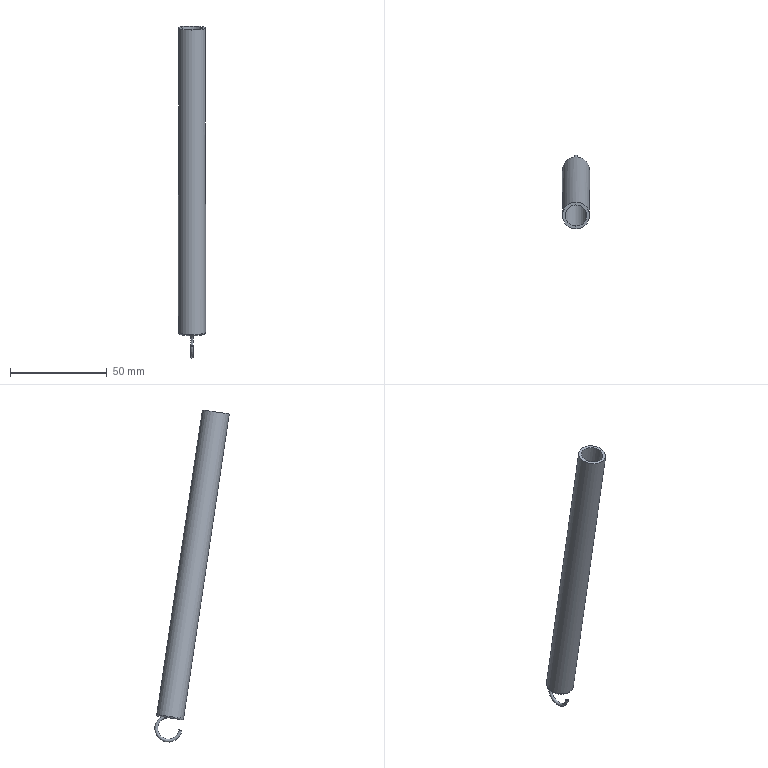Part | NX | features solid 2 | 1 solid | 7 faces | box 14 x 38.402 x 171.464 mm | volume 9463 mm3 | cylinder 3 | torus 2 | plane 2 | commonest cylinder face diameters 1.5 x1 11 x1 14 x1
STEP:
#1=CARTESIAN_POINT('',(-73.065,137.352,-927.911));
#2=VERTEX_POINT('',#1);
#3=CARTESIAN_POINT('',(-80.065,137.352,-927.911));
#4=DIRECTION('',(0.,-0.1481,0.989));
#5=DIRECTION('',(1.,0.,0.));
#6=AXIS2_PLACEMENT_3D('',#3,#4,#5);
#7=CIRCLE('',#6,7.);
#8=EDGE_CURVE('',#2,#2,#7,.T.);
#9=ORIENTED_EDGE('',*,*,#8,.T.);
#10=EDGE_LOOP('',(#9));
#11=FACE_BOUND('',#10,.T.);
#12=CARTESIAN_POINT('',(-80.065,106.877,-771.702));
#13=VERTEX_POINT('',#12);
#14=CARTESIAN_POINT('',(-80.065,113.799,-770.665));
#15=DIRECTION('',(0.,-0.1481,0.989));
#16=DIRECTION('',(0.,-0.989,-0.1481));
#17=AXIS2_PLACEMENT_3D('',#14,#15,#16);
#18=CIRCLE('',#17,7.);
#19=EDGE_CURVE('',#13,#13,#18,.F.);
#20=ORIENTED_EDGE('',*,*,#19,.T.);
#21=EDGE_LOOP('',(#20));
#22=FACE_BOUND('',#21,.T.);
#23=CARTESIAN_POINT('',(-80.065,101.766,-690.33));
#24=DIRECTION('',(0.,0.1481,-0.989));
#25=DIRECTION('',(-1.,0.,0.));
#26=AXIS2_PLACEMENT_3D('',#23,#24,#25);
#27=CYLINDRICAL_SURFACE('',#26,7.);
#28=ADVANCED_FACE('',(#11,#22),#27,.T.);
#29=CARTESIAN_POINT('',(-79.315,131.964,-928.718));
#30=VERTEX_POINT('',#29);
#31=CARTESIAN_POINT('',(-80.815,131.964,-928.718));
#32=VERTEX_POINT('',#31);
#33=CARTESIAN_POINT('',(-80.065,137.352,-927.911));
#34=DIRECTION('',(0.,-0.1481,0.989));
#35=DIRECTION('',(-1.,0.,0.));
#36=AXIS2_PLACEMENT_3D('',#33,#34,#35);
#37=CIRCLE('',#36,5.5);
#38=EDGE_CURVE('',#30,#32,#37,.T.);
#39=ORIENTED_EDGE('',*,*,#38,.F.);
#40=CARTESIAN_POINT('',(-80.815,131.964,-928.718));
#41=CARTESIAN_POINT('',(-80.815,131.905,-928.325));
#42=CARTESIAN_POINT('',(-80.066,131.699,-927.642));
#43=CARTESIAN_POINT('',(-79.315,131.905,-928.325));
#44=CARTESIAN_POINT('',(-79.315,131.964,-928.718));
#45=B_SPLINE_CURVE_WITH_KNOTS('',3,(#40,#41,#42,#43,#44),.UNSPECIFIED.,.F.,.F.,(4,1,4),(0.,0.001174,0.002347),.UNSPECIFIED.);
#46=EDGE_CURVE('',#32,#30,#45,.T.);
#47=ORIENTED_EDGE('',*,*,#46,.F.);
#48=EDGE_LOOP('',(#39,#47));
#49=FACE_BOUND('',#48,.T.);
#50=CARTESIAN_POINT('',(-80.065,108.36,-771.48));
#51=VERTEX_POINT('',#50);
#52=CARTESIAN_POINT('',(-80.065,113.799,-770.665));
#53=DIRECTION('',(0.,-0.1481,0.989));
#54=DIRECTION('',(0.,-0.989,-0.1481));
#55=AXIS2_PLACEMENT_3D('',#52,#53,#54);
#56=CIRCLE('',#55,5.5);
#57=EDGE_CURVE('',#51,#51,#56,.T.);
#58=ORIENTED_EDGE('',*,*,#57,.T.);
#59=EDGE_LOOP('',(#58));
#60=FACE_BOUND('',#59,.T.);
#61=CARTESIAN_POINT('',(-80.065,101.766,-690.33));
#62=DIRECTION('',(0.,0.1481,-0.989));
#63=DIRECTION('',(-1.,0.,0.));
#64=AXIS2_PLACEMENT_3D('',#61,#62,#63);
#65=CYLINDRICAL_SURFACE('',#64,5.5);
#66=ADVANCED_FACE('',(#49,#60),#65,.F.);
#67=ORIENTED_EDGE('',*,*,#38,.T.);
#68=CARTESIAN_POINT('',(-80.065,131.283,-929.578));
#69=VERTEX_POINT('',#68);
#70=CARTESIAN_POINT('',(-80.815,131.964,-928.718));
#71=CARTESIAN_POINT('',(-80.815,132.001,-928.962));
#72=CARTESIAN_POINT('',(-80.572,131.784,-929.4));
#73=CARTESIAN_POINT('',(-80.237,131.452,-929.553));
#74=CARTESIAN_POINT('',(-80.065,131.283,-929.578));
#75=B_SPLINE_CURVE_WITH_KNOTS('',3,(#70,#71,#72,#73,#74),.UNSPECIFIED.,.F.,.F.,(4,1,4),(0.,0.0007272,0.001454),.UNSPECIFIED.);
#76=EDGE_CURVE('',#32,#69,#75,.T.);
#77=ORIENTED_EDGE('',*,*,#76,.T.);
#78=CARTESIAN_POINT('',(-79.315,131.964,-928.718));
#79=CARTESIAN_POINT('',(-79.315,132.001,-928.962));
#80=CARTESIAN_POINT('',(-79.558,131.784,-929.4));
#81=CARTESIAN_POINT('',(-79.894,131.452,-929.553));
#82=CARTESIAN_POINT('',(-80.065,131.283,-929.578));
#83=B_SPLINE_CURVE_WITH_KNOTS('',3,(#78,#79,#80,#81,#82),.UNSPECIFIED.,.F.,.F.,(4,1,4),(0.,0.0007272,0.001454),.UNSPECIFIED.);
#84=EDGE_CURVE('',#69,#30,#83,.F.);
#85=ORIENTED_EDGE('',*,*,#84,.T.);
#86=EDGE_LOOP('',(#67,#77,#85));
#87=FACE_BOUND('',#86,.T.);
#88=ORIENTED_EDGE('',*,*,#8,.F.);
#89=EDGE_LOOP('',(#88));
#90=FACE_BOUND('',#89,.T.);
#91=CARTESIAN_POINT('',(-80.065,137.352,-927.911));
#92=DIRECTION('',(0.,-0.1481,0.989));
#93=DIRECTION('',(-1.,0.,0.));
#94=AXIS2_PLACEMENT_3D('',#91,#92,#93);
#95=TOROIDAL_SURFACE('',#94,6.25,0.75);
#96=ADVANCED_FACE('',(#87,#90),#95,.T.);
#97=CARTESIAN_POINT('',(-80.065,131.339,-935.008));
#98=VERTEX_POINT('',#97);
#99=CARTESIAN_POINT('',(-80.065,132.082,-934.91));
#100=DIRECTION('',(0.,0.1309,-0.9914));
#101=DIRECTION('',(0.,-0.9914,-0.1309));
#102=AXIS2_PLACEMENT_3D('',#99,#100,#101);
#103=CIRCLE('',#102,0.75);
#104=EDGE_CURVE('',#98,#98,#103,.T.);
#105=ORIENTED_EDGE('',*,*,#104,.T.);
#106=EDGE_LOOP('',(#105));
#107=FACE_BOUND('',#106,.T.);
#108=CARTESIAN_POINT('',(-79.315,137.352,-927.911));
#109=VERTEX_POINT('',#108);
#110=CARTESIAN_POINT('',(-80.065,137.352,-927.911));
#111=DIRECTION('',(0.,-0.989,-0.1481));
#112=DIRECTION('',(1.,0.,0.));
#113=AXIS2_PLACEMENT_3D('',#110,#111,#112);
#114=CIRCLE('',#113,0.75);
#115=EDGE_CURVE('',#109,#109,#114,.T.);
#116=ORIENTED_EDGE('',*,*,#115,.F.);
#117=EDGE_LOOP('',(#116));
#118=FACE_BOUND('',#117,.T.);
#119=CARTESIAN_POINT('',(-80.065,138.278,-934.092));
#120=DIRECTION('',(-1.,0.,0.));
#121=DIRECTION('',(0.,0.1481,-0.989));
#122=AXIS2_PLACEMENT_3D('',#119,#120,#121);
#123=TOROIDAL_SURFACE('',#122,6.25,0.75);
#124=ADVANCED_FACE('',(#107,#118),#123,.T.);
#125=ORIENTED_EDGE('',*,*,#115,.T.);
#126=EDGE_LOOP('',(#125));
#127=FACE_BOUND('',#126,.T.);
#128=ORIENTED_EDGE('',*,*,#76,.F.);
#129=ORIENTED_EDGE('',*,*,#46,.T.);
#130=ORIENTED_EDGE('',*,*,#84,.F.);
#131=EDGE_LOOP('',(#128,#129,#130));
#132=FACE_BOUND('',#131,.T.);
#133=CARTESIAN_POINT('',(-80.065,134.262,-928.374));
#134=DIRECTION('',(0.,0.989,0.1481));
#135=DIRECTION('',(-1.,0.,0.));
#136=AXIS2_PLACEMENT_3D('',#133,#134,#135);
#137=CYLINDRICAL_SURFACE('',#136,0.75);
#138=ADVANCED_FACE('',(#127,#132),#137,.T.);
#139=ORIENTED_EDGE('',*,*,#104,.F.);
#140=EDGE_LOOP('',(#139));
#141=FACE_BOUND('',#140,.T.);
#142=CARTESIAN_POINT('',(-80.065,132.082,-934.91));
#143=DIRECTION('',(0.,0.1309,-0.9914));
#144=DIRECTION('',(0.,0.9914,0.1309));
#145=AXIS2_PLACEMENT_3D('',#142,#143,#144);
#146=PLANE('',#145);
#147=ADVANCED_FACE('',(#141),#146,.F.);
#148=ORIENTED_EDGE('',*,*,#19,.F.);
#149=EDGE_LOOP('',(#148));
#150=FACE_BOUND('',#149,.T.);
#151=ORIENTED_EDGE('',*,*,#57,.F.);
#152=EDGE_LOOP('',(#151));
#153=FACE_BOUND('',#152,.T.);
#154=CARTESIAN_POINT('',(-80.065,113.799,-770.665));
#155=DIRECTION('',(0.,-0.1481,0.989));
#156=DIRECTION('',(0.,-0.989,-0.1481));
#157=AXIS2_PLACEMENT_3D('',#154,#155,#156);
#158=PLANE('',#157);
#159=ADVANCED_FACE('',(#150,#153),#158,.T.);
#160=CLOSED_SHELL('',(#28,#66,#96,#124,#138,#147,#159));
#161=MANIFOLD_SOLID_BREP('',#160);
#162=(LENGTH_UNIT()NAMED_UNIT(*)SI_UNIT(.MILLI.,.METRE.));
#163=UNCERTAINTY_MEASURE_WITH_UNIT(LENGTH_MEASURE(0.0508),#162,'','');
#164=(NAMED_UNIT(*)PLANE_ANGLE_UNIT()SI_UNIT($,.RADIAN.));
#165=(NAMED_UNIT(*)SI_UNIT($,.STERADIAN.)SOLID_ANGLE_UNIT());
#166=(GEOMETRIC_REPRESENTATION_CONTEXT(3)GLOBAL_UNCERTAINTY_ASSIGNED_CONTEXT((#163))GLOBAL_UNIT_ASSIGNED_CONTEXT((#162,#164,#165))REPRESENTATION_CONTEXT('',''));
#167=ADVANCED_BREP_SHAPE_REPRESENTATION('',(#161),#166);